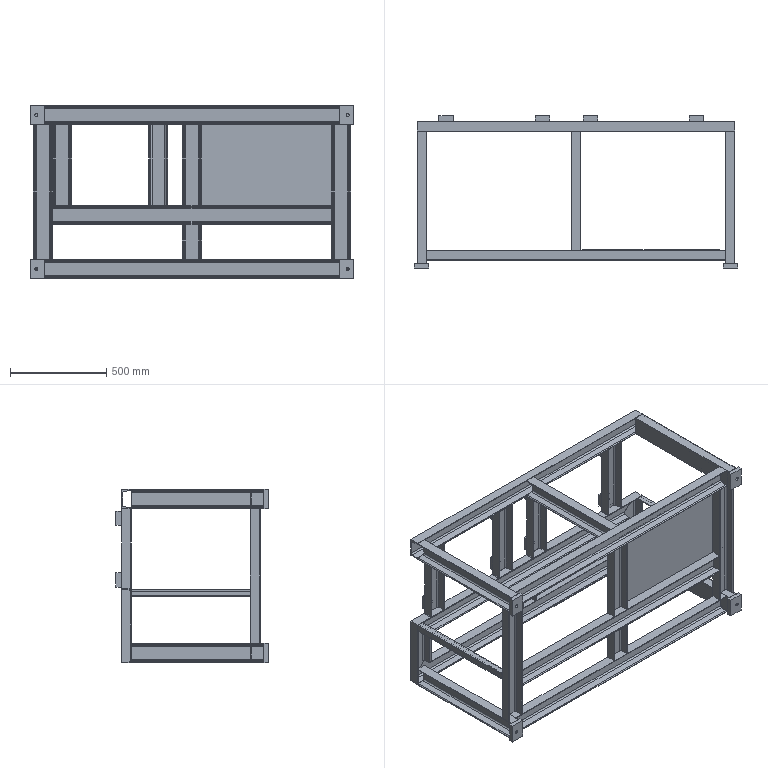Part | STEP file | OP10-001_base frame(Default_As Machined_) | 61 solids | 548 faces | box 1680 x 792 x 900 mm | volume 25499684 mm3 | plane 430 | cylinder 118 | commonest cylinder face diameters 16 x68 9 x44 10 x6